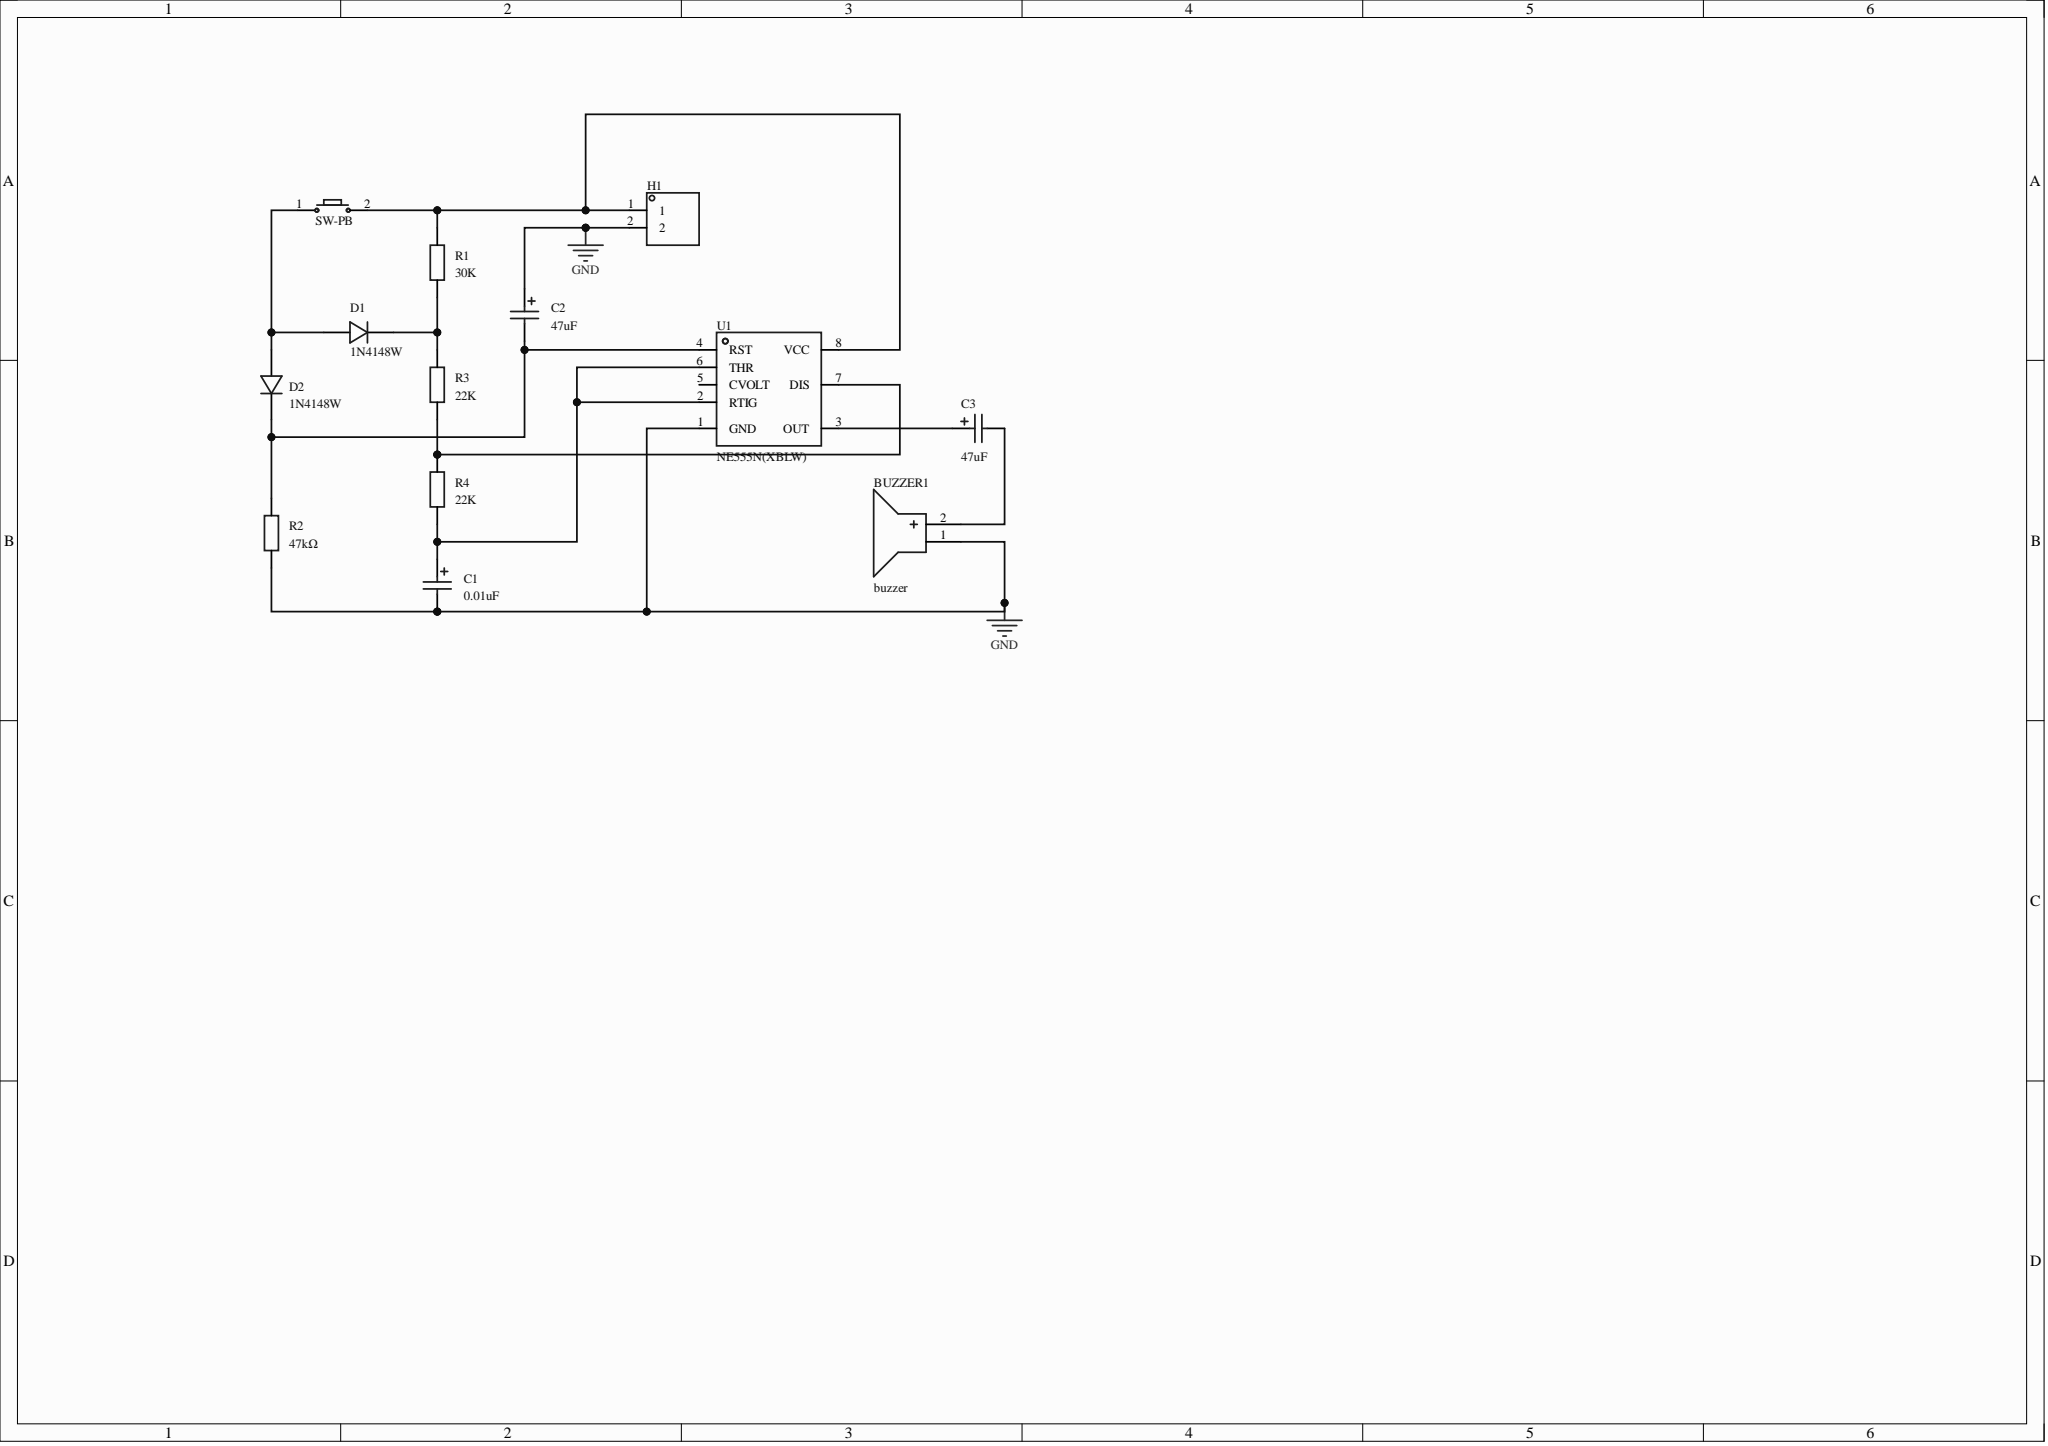Circuit board | Altium Designer | 13 parts | 9 nets
Bill of materials:
Comment,Description,Designator,Footprint,LibRef,Quantity
"buzzer","","BUZZER1","BUZ-TH_BD12.0-P6.00-D0.9-RD","buzzer","1"
"0.01uF","","C1","C_Ele_SMD_3x5.4mm","C_Ele_SMD_3x5.4mm","1"
"47uF","","C2, C3","C_Ele_SMD_3x5.4mm","C_Ele_SMD_3x5.4mm","2"
"1N4148W","Diode configuration: Independent; forward voltage (Vf): 1.25V@150mA; DC reverse withstand voltage (Vr): 100V; rectified current: 150mA; reverse recovery time (Trr): 4ns;","D1, D2","SOD-323_L1.8-W1.3-LS2.5-RD","1N4148WS_C2128","2"
"","","H1","HDR-TH_2P-P2.54-V-M-1","HDR-M_2.54_1x2P","1"
"30K","","R1","R0603","Res_0603","1"
"47kΩ","","R2","Res_1/8W","Res_AXIAL-1/8W","1"
"22K","","R3, R4","R0603","Res_0603","2"
"","","SW-PB","Key_SMD_3x4x2","Key_SMD_3x4x2","1"
"NE555N(XBLW)","Timer, time-base timer","U1","PDIP-8_L9.5-W6.4-P2.54-LS7.6-BL","NE555N(XBLW)","1"
Netlist (Protel format):
[
BUZZER1
BUZ-TH_BD12.0-P6.00-D0.9-RD
buzzer



]
[
C1
C_Ele_SMD_3x5.4mm
0.01uF



]
[
C2
C_Ele_SMD_3x5.4mm
47uF



]
[
C3
C_Ele_SMD_3x5.4mm
47uF



]
[
D1
SOD-323_L1.8-W1.3-LS2.5-RD
1N4148W



]
[
D2
SOD-323_L1.8-W1.3-LS2.5-RD
1N4148W



]
[
H1
HDR-TH_2P-P2.54-V-M-1




]
[
R1
R0603
30K



]
[
R2
Res_1/8W
47kΩ



]
[
R3
R0603
22K



]
[
R4
R0603
22K



]
[
SW-PB
Key_SMD_3x4x2




]
[
U1
PDIP-8_L9.5-W6.4-P2.54-LS7.6-BL
NE555N(XBLW)



]
(
NetR3_1
R3-1
R4-2
U1-7
)
(
NetH1_1
H1-1
R1-2
SW-PB-2
U1-8
)
(
NetD1_2
D1-2
D2-2
SW-PB-1
)
(
NetD1_1
D1-1
R1-1
R3-2
)
(
NetC3_1
C3-1
U1-3
)
(
NetC2_2
C2-2
D2-1
R2-2
U1-4
)
(
NetC1_1
C1-1
R4-1
U1-2
U1-6
)
(
NetBUZZER1_2
BUZZER1-2
C3-2
)
(
GND
BUZZER1-1
C1-2
C2-1
H1-2
R2-1
U1-1
)